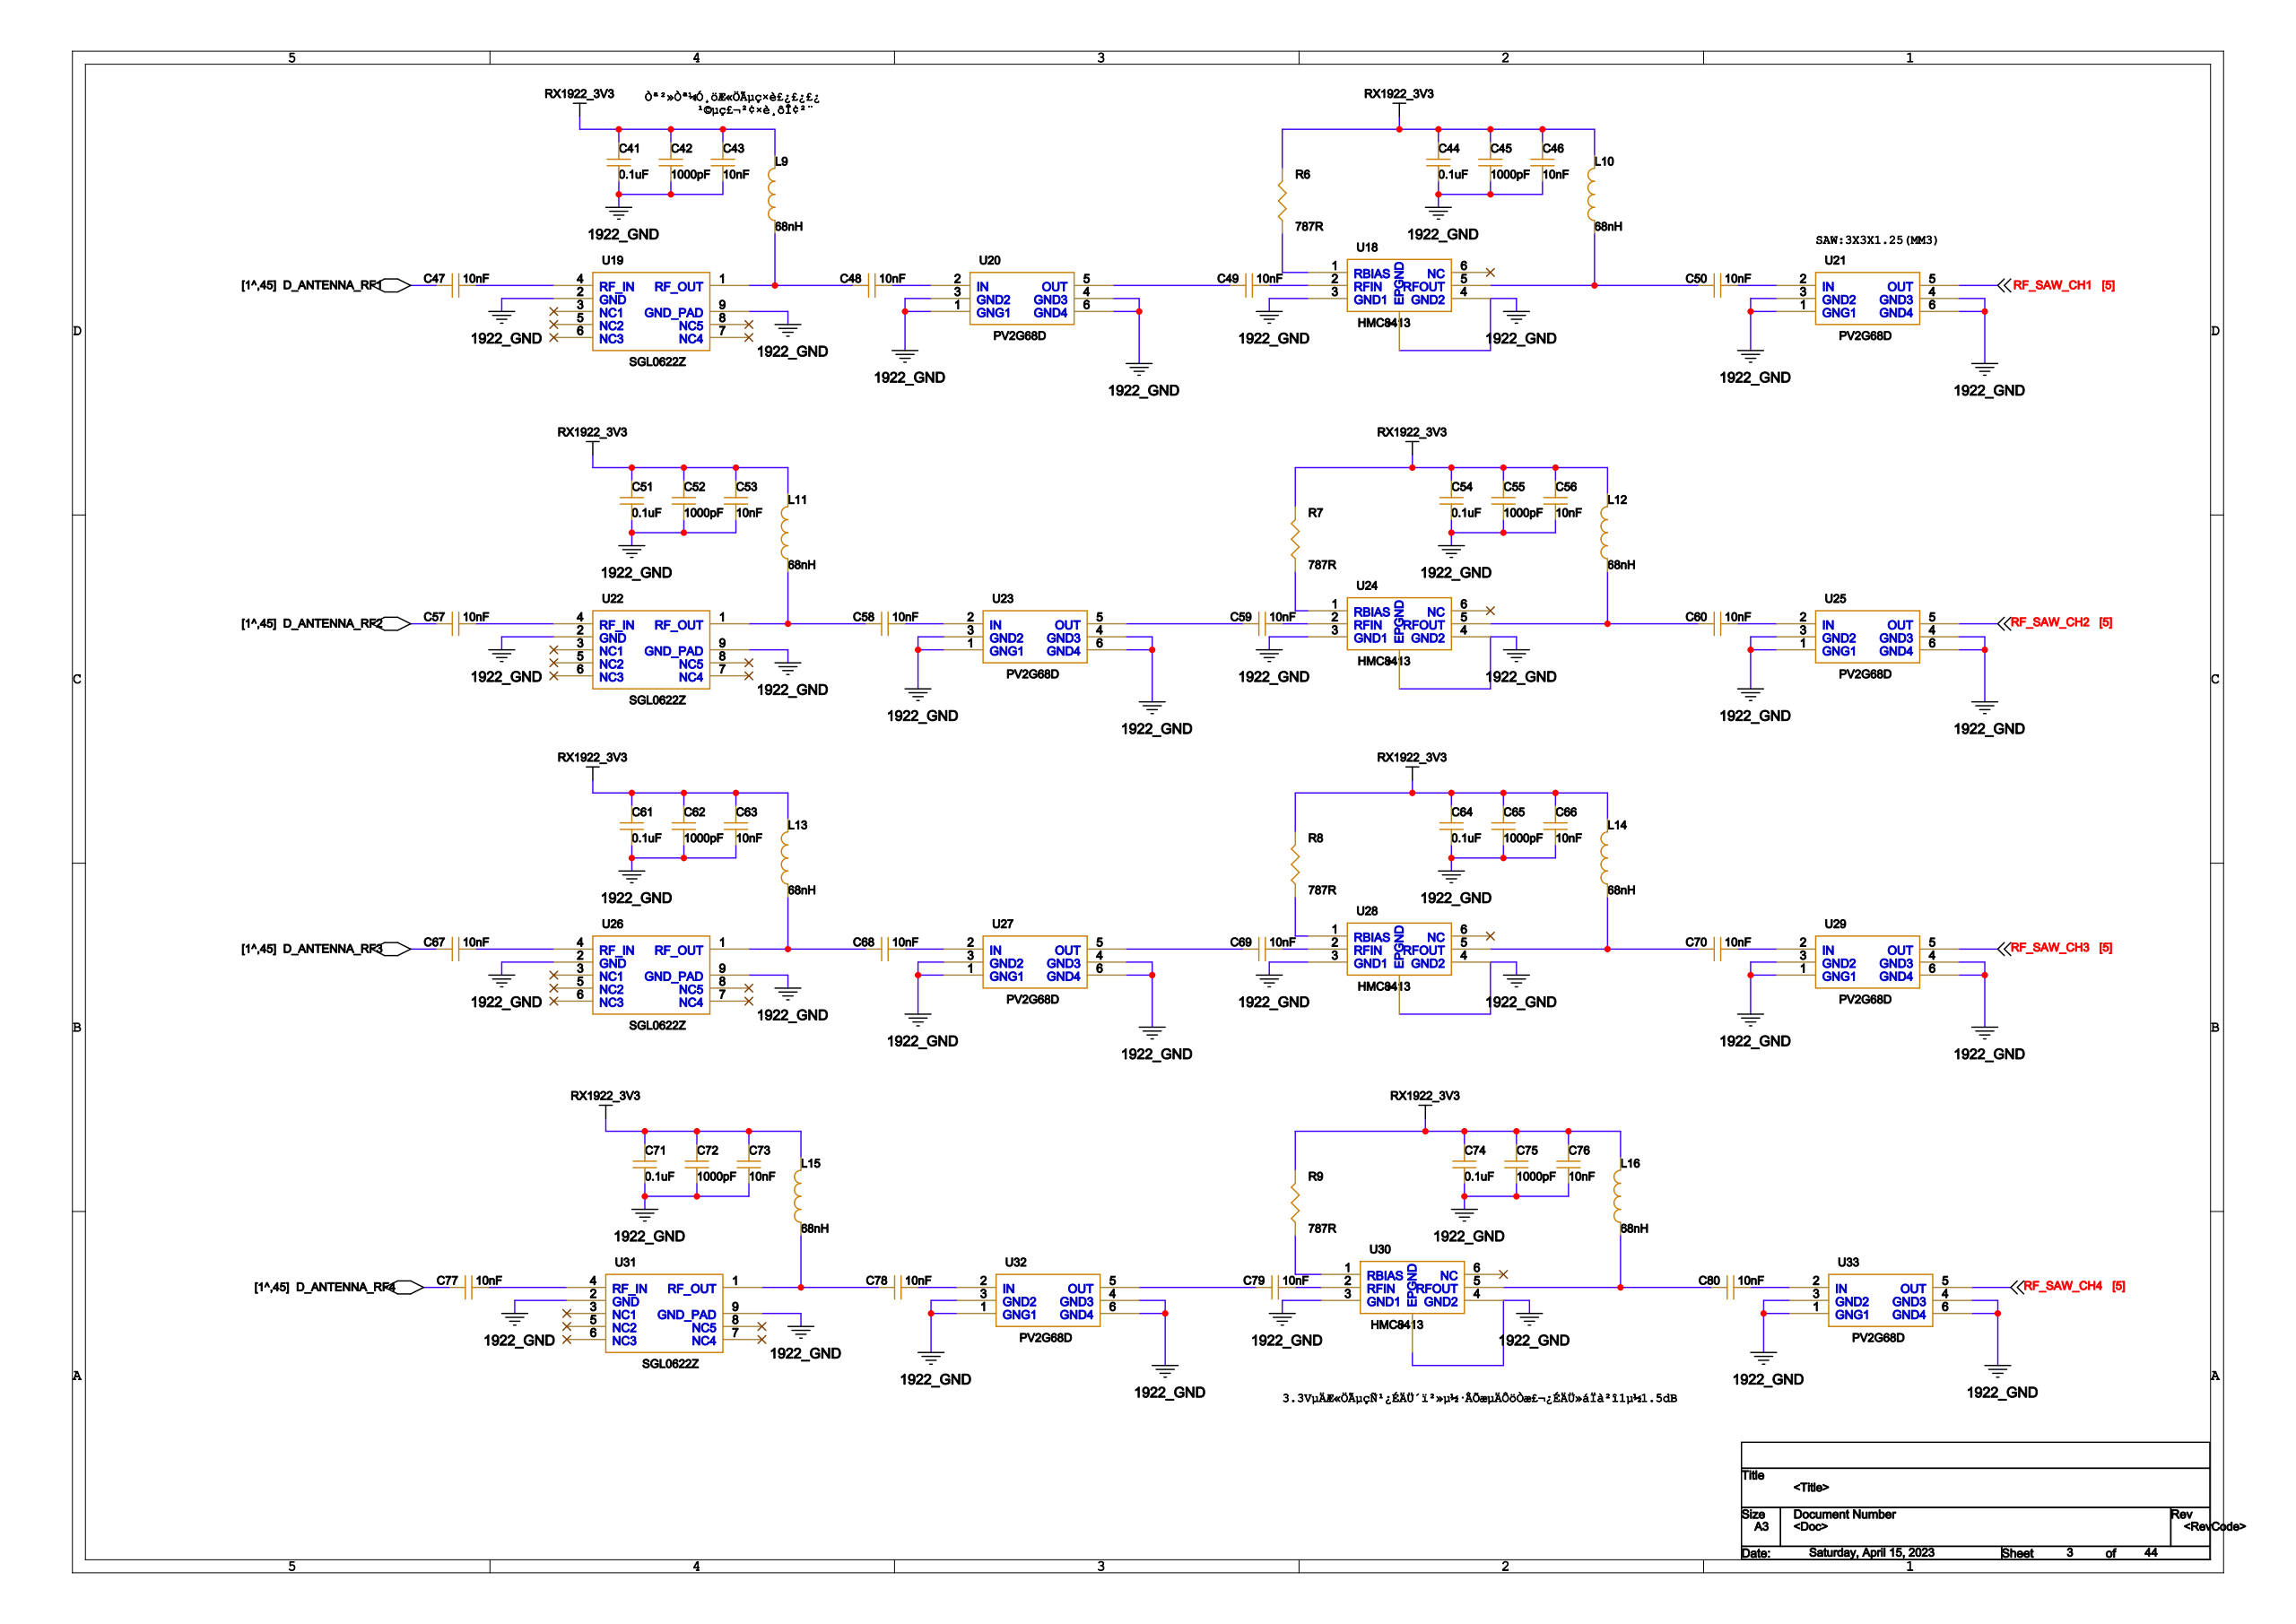Circuit board | Cadence Allegro | 1034 parts | 912 nets | one sheet of the schematic
Parts on this sheet (reference | value | footprint):
C41 | 0.1uF | C0402
C42 | 1000pF | C0402
C43 | 10nF | C0402
C44 | 0.1uF | C0402
C45 | 1000pF | C0402
C46 | 10nF | C0402
C47 | 10nF | C0402
C48 | 10nF | C0402
C49 | 10nF | C0402
C50 | 10nF | C0402
C51 | 0.1uF | C0402
C52 | 1000pF | C0402
C53 | 10nF | C0402
C54 | 0.1uF | C0402
C55 | 1000pF | C0402
C56 | 10nF | C0402
C57 | 10nF | C0402
C58 | 10nF | C0402
C59 | 10nF | C0402
C60 | 10nF | C0402
C61 | 0.1uF | C0402
C62 | 1000pF | C0402
C63 | 10nF | C0402
C64 | 0.1uF | C0402
C65 | 1000pF | C0402
C66 | 10nF | C0402
C67 | 10nF | C0402
C68 | 10nF | C0402
C69 | 10nF | C0402
C70 | 10nF | C0402
C71 | 0.1uF | C0402
C72 | 1000pF | C0402
C73 | 10nF | C0402
C74 | 0.1uF | C0402
C75 | 1000pF | C0402
C76 | 10nF | C0402
C77 | 10nF | C0402
C78 | 10nF | C0402
C79 | 10nF | C0402
C80 | 10nF | C0402
L9 | 68nH | L0402
L10 | 68nH | L0402
L11 | 68nH | L0402
L12 | 68nH | L0402
L13 | 68nH | L0402
L14 | 68nH | L0402
L15 | 68nH | L0402
L16 | 68nH | L0402
R6 | 787R | R0402
R7 | 787R | R0402
R8 | 787R | R0402
R9 | 787R | R0402
U18 | HMC8413 | HMC8413_LFCSP
U19 | SGL0622Z | GL0622_DFN
U20 | PV2G68D | G68D_DCC6C
U21 | PV2G68D | G68D_DCC6C
U22 | SGL0622Z | GL0622_DFN
U23 | PV2G68D | G68D_DCC6C
U24 | HMC8413 | HMC8413_LFCSP
U25 | PV2G68D | G68D_DCC6C
U26 | SGL0622Z | GL0622_DFN
U27 | PV2G68D | G68D_DCC6C
U28 | HMC8413 | HMC8413_LFCSP
U29 | PV2G68D | G68D_DCC6C
U30 | HMC8413 | HMC8413_LFCSP
U31 | SGL0622Z | GL0622_DFN
U32 | PV2G68D | G68D_DCC6C
U33 | PV2G68D | G68D_DCC6C
Nets of these parts (net: part-pin ...):
RF_SAW_CH1_D2: U21-5
RF_SAW_CH2_D2: U25-5
RF_SAW_CH3_D2: U29-5
RF_SAW_CH4_D2: U33-5
1922_GND: C41-1 C42-1 C43-1 C44-1 C45-1 C46-1 C51-1 C52-1 C53-1 C54-1 C55-1 C56-1 C61-1 C62-1 C63-1 C64-1 C65-1 C66-1 C71-1 C72-1 C73-1 C74-1 C75-1 C76-1 U18-3 U18-4 U18-7 U19-2 U19-9 U20-1 U20-3 U20-4 U20-6 U21-1 U21-3 U21-4 U21-6 U22-2 U22-9 U23-1 U23-3 U23-4 U23-6 U24-3 U24-4 U24-7 U25-1 U25-3 U25-4 U25-6 U26-2 U26-9 U27-1 U27-3 U27-4 U27-6 U28-3 U28-4 U28-7 U29-1 U29-3 U29-4 U29-6 U30-3 U30-4 U30-7 U31-2 U31-9 U32-1 U32-3 U32-4 U32-6 U33-1 U33-3 U33-4 U33-6
PWR1922_3V3_2: C41-2 C42-2 C43-2 C44-2 C45-2 C46-2 C51-2 C52-2 C53-2 C54-2 C55-2 C56-2 C61-2 C62-2 C63-2 C64-2 C65-2 C66-2 C71-2 C72-2 C73-2 C74-2 C75-2 C76-2 L9-2 L10-2 L11-2 L12-2 L13-2 L14-2 L15-2 L16-2 R6-2 R7-2 R8-2 R9-2
N14178364_D2: R6-1 U18-1
N14160942_D2: C49-2 U18-2
N14157205_D2: C50-1 L10-1 U18-5
N14181093_D2: R7-1 U24-1
N14161005_D2: C59-2 U24-2
N14157931_D2: C60-1 L12-1 U24-5
N14181388_D2: R8-1 U28-1
N14161069_D2: C69-2 U28-2
N14158707_D2: C70-1 L14-1 U28-5
N14181679_D2: R9-1 U30-1
N14161133_D2: C79-2 U30-2
N14159525_D2: C80-1 L16-1 U30-5
N185273: C47-1
N14090512_D2: C47-2 U19-4
N14147824_D2: C48-1 L9-1 U19-1
N14165389_D2: C48-2 U20-2
N14165393_D2: C49-1 U20-5
N14088748_D2: C50-2 U21-2
N185289: C57-1
N14091229_D2: C57-2 U22-4
N14147816_D2: C58-1 L11-1 U22-1
N14166037_D2: C58-2 U23-2
N14166041_D2: C59-1 U23-5
N14089401_D2: C60-2 U25-2
N185301: C67-1
N14091629_D2: C67-2 U26-4
N14147828_D2: C68-1 L13-1 U26-1
N14166455_D2: C68-2 U27-2
N14166459_D2: C69-1 U27-5
N14089671_D2: C70-2 U29-2
N185313: C77-1
N14092049_D2: C77-2 U31-4
N14147820_D2: C78-1 L15-1 U31-1
N14166887_D2: C78-2 U32-2
N14166891_D2: C79-1 U32-5
N14089951_D2: C80-2 U33-2